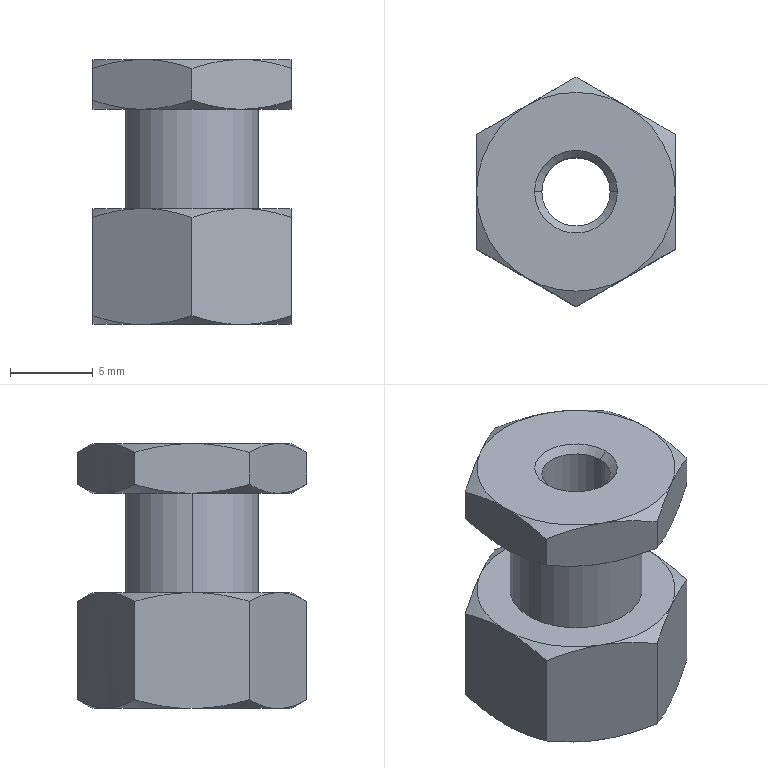Part | SolidWorks | features BaseBody 1 | 1 solid | 48 faces | box 12 x 13.856 x 16 mm | volume 1324 mm3 | cone 28 | plane 16 | cylinder 4 | commonest cylinder face diameters 4.134 x2 8 x2